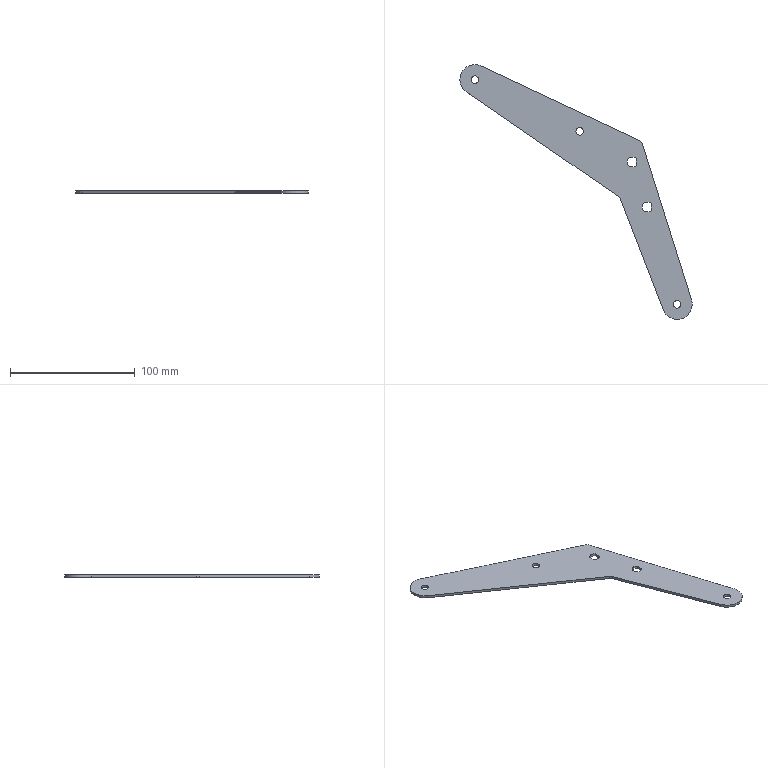Part | STEP file | 1 solid | 21 faces | box 186 x 204 x 2 mm | volume 17144 mm3 | cylinder 13 | plane 8 | commonest cylinder face diameters 6 x6 24 x3 8 x2 10 x2